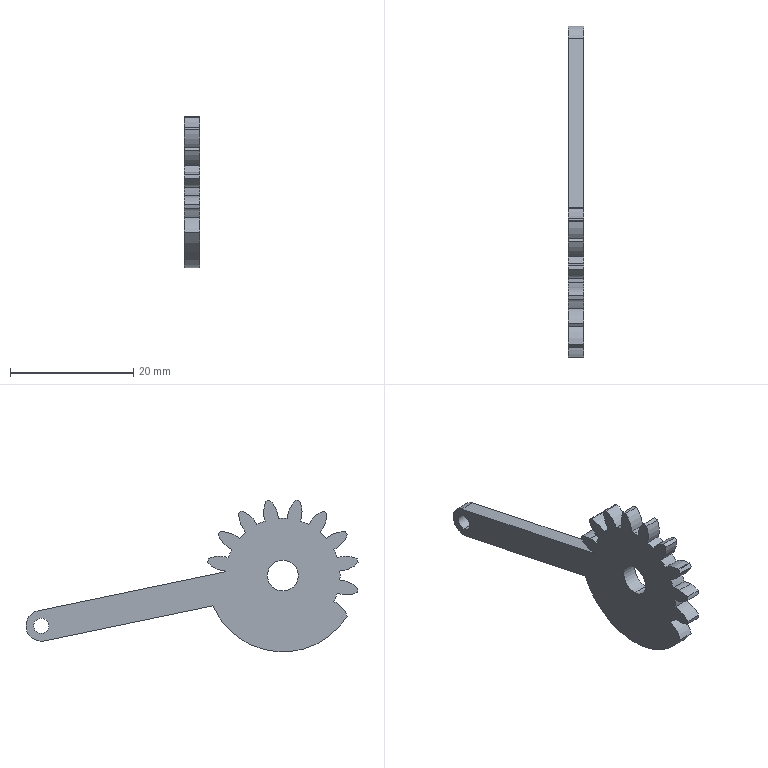Part | SolidWorks | features ICE 4, MoveCopyBody 1, Stock 1 | 1 solid | 54 faces | box 2.5 x 53.856 x 24.571 mm | volume 1339 mm3 | cylinder 50 | plane 4 | commonest cylinder face diameters 8.8 x23 18.561 x11 24.75 x10 2.5 x2 4.999 x2 5 x2